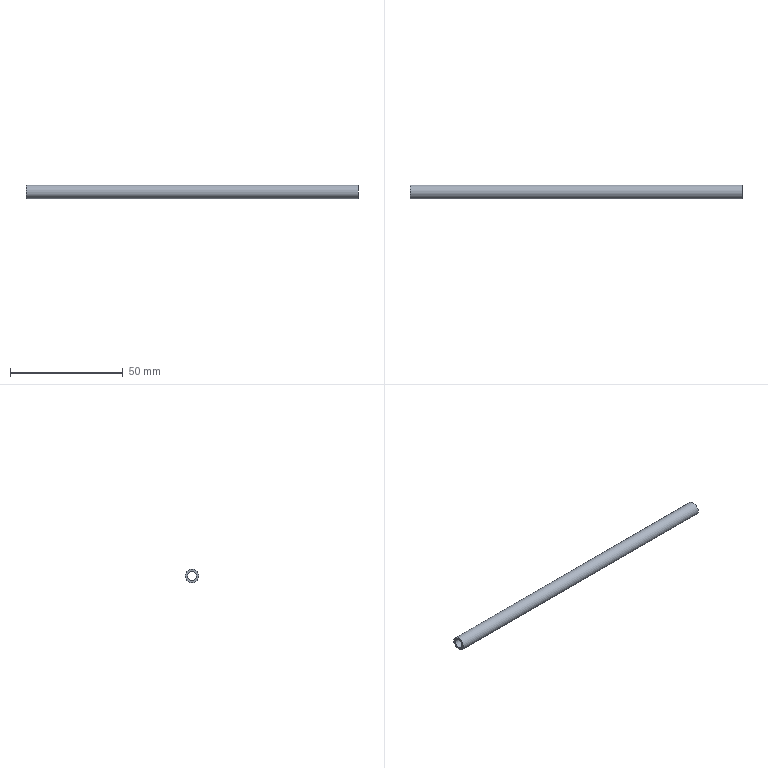Part | NX | features solid 2 | 1 solid | 4 faces | box 147.125 x 6 x 6 mm | volume 2311 mm3 | cylinder 2 | plane 2 | commonest cylinder face diameters 4 x1 6 x1
STEP:
#1=CARTESIAN_POINT('',(257.125,39.,347.));
#2=VERTEX_POINT('',#1);
#3=CARTESIAN_POINT('',(257.125,41.,347.));
#4=DIRECTION('',(-1.,0.,0.));
#5=DIRECTION('',(0.,-1.,0.));
#6=AXIS2_PLACEMENT_3D('',#3,#4,#5);
#7=CIRCLE('',#6,2.);
#8=EDGE_CURVE('',#2,#2,#7,.T.);
#9=ORIENTED_EDGE('',*,*,#8,.F.);
#10=EDGE_LOOP('',(#9));
#11=FACE_BOUND('',#10,.T.);
#12=CARTESIAN_POINT('',(110.,39.,347.));
#13=VERTEX_POINT('',#12);
#14=CARTESIAN_POINT('',(110.,41.,347.));
#15=DIRECTION('',(-1.,0.,0.));
#16=DIRECTION('',(0.,-1.,0.));
#17=AXIS2_PLACEMENT_3D('',#14,#15,#16);
#18=CIRCLE('',#17,2.);
#19=EDGE_CURVE('',#13,#13,#18,.T.);
#20=ORIENTED_EDGE('',*,*,#19,.T.);
#21=EDGE_LOOP('',(#20));
#22=FACE_BOUND('',#21,.T.);
#23=CARTESIAN_POINT('',(216.176,41.,347.));
#24=DIRECTION('',(1.,0.,0.));
#25=DIRECTION('',(0.,1.,0.));
#26=AXIS2_PLACEMENT_3D('',#23,#24,#25);
#27=CYLINDRICAL_SURFACE('',#26,2.);
#28=ADVANCED_FACE('',(#11,#22),#27,.F.);
#29=CARTESIAN_POINT('',(257.125,38.,347.));
#30=VERTEX_POINT('',#29);
#31=CARTESIAN_POINT('',(257.125,41.,347.));
#32=DIRECTION('',(-1.,0.,0.));
#33=DIRECTION('',(0.,-1.,0.));
#34=AXIS2_PLACEMENT_3D('',#31,#32,#33);
#35=CIRCLE('',#34,3.);
#36=EDGE_CURVE('',#30,#30,#35,.T.);
#37=ORIENTED_EDGE('',*,*,#36,.T.);
#38=EDGE_LOOP('',(#37));
#39=FACE_BOUND('',#38,.T.);
#40=CARTESIAN_POINT('',(110.,38.,347.));
#41=VERTEX_POINT('',#40);
#42=CARTESIAN_POINT('',(110.,41.,347.));
#43=DIRECTION('',(-1.,0.,0.));
#44=DIRECTION('',(0.,-1.,0.));
#45=AXIS2_PLACEMENT_3D('',#42,#43,#44);
#46=CIRCLE('',#45,3.);
#47=EDGE_CURVE('',#41,#41,#46,.T.);
#48=ORIENTED_EDGE('',*,*,#47,.F.);
#49=EDGE_LOOP('',(#48));
#50=FACE_BOUND('',#49,.T.);
#51=CARTESIAN_POINT('',(216.176,41.,347.));
#52=DIRECTION('',(1.,0.,0.));
#53=DIRECTION('',(0.,1.,0.));
#54=AXIS2_PLACEMENT_3D('',#51,#52,#53);
#55=CYLINDRICAL_SURFACE('',#54,3.);
#56=ADVANCED_FACE('',(#39,#50),#55,.T.);
#57=ORIENTED_EDGE('',*,*,#8,.T.);
#58=EDGE_LOOP('',(#57));
#59=FACE_BOUND('',#58,.T.);
#60=ORIENTED_EDGE('',*,*,#36,.F.);
#61=EDGE_LOOP('',(#60));
#62=FACE_BOUND('',#61,.T.);
#63=CARTESIAN_POINT('',(257.125,80.83,185.));
#64=DIRECTION('',(-1.,0.,0.));
#65=DIRECTION('',(0.,-1.,0.));
#66=AXIS2_PLACEMENT_3D('',#63,#64,#65);
#67=PLANE('',#66);
#68=ADVANCED_FACE('',(#59,#62),#67,.F.);
#69=ORIENTED_EDGE('',*,*,#19,.F.);
#70=EDGE_LOOP('',(#69));
#71=FACE_BOUND('',#70,.T.);
#72=ORIENTED_EDGE('',*,*,#47,.T.);
#73=EDGE_LOOP('',(#72));
#74=FACE_BOUND('',#73,.T.);
#75=CARTESIAN_POINT('',(110.,35.,347.));
#76=DIRECTION('',(-1.,0.,0.));
#77=DIRECTION('',(0.,-1.,0.));
#78=AXIS2_PLACEMENT_3D('',#75,#76,#77);
#79=PLANE('',#78);
#80=ADVANCED_FACE('',(#71,#74),#79,.T.);
#81=CLOSED_SHELL('',(#28,#56,#68,#80));
#82=MANIFOLD_SOLID_BREP('',#81);
#83=(LENGTH_UNIT()NAMED_UNIT(*)SI_UNIT(.MILLI.,.METRE.));
#84=UNCERTAINTY_MEASURE_WITH_UNIT(LENGTH_MEASURE(0.00001),#83,'','');
#85=(NAMED_UNIT(*)PLANE_ANGLE_UNIT()SI_UNIT($,.RADIAN.));
#86=(NAMED_UNIT(*)SI_UNIT($,.STERADIAN.)SOLID_ANGLE_UNIT());
#87=(GEOMETRIC_REPRESENTATION_CONTEXT(3)GLOBAL_UNCERTAINTY_ASSIGNED_CONTEXT((#84))GLOBAL_UNIT_ASSIGNED_CONTEXT((#83,#85,#86))REPRESENTATION_CONTEXT('',''));
#88=ADVANCED_BREP_SHAPE_REPRESENTATION('',(#82),#87);